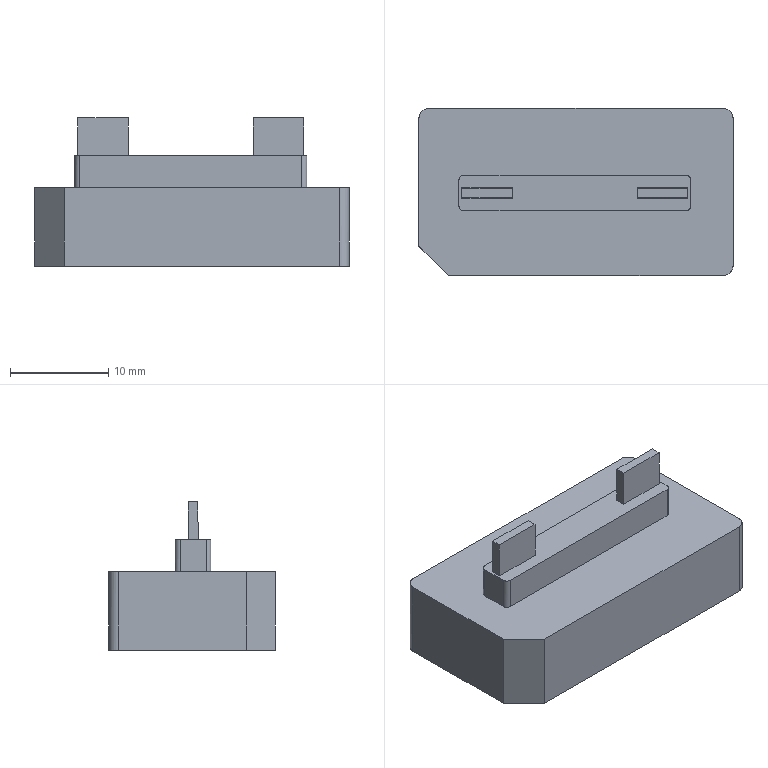NC program | PowerMill | posted by the shop | part box 32 x 17 x 15.109 mm
Lines 3804 to 5363 of 35413:
( TOOL ID   D3_2_1 )
( TOOL DIA. 3. TIP RAD 0 LENGTH 62.2 )
( Z = -7.279 )
T10 M6
T13
G91 G28 Z0
G0 G90 G54
M08
S18000 M3
X0 Y0 M8
G43 Z10.799 H10
X12.217 Y-2.308
Z.814
G1 Z-.386 F1200
X12.204 Y-2.248 F2000
X12.183 Y-2.19
X12.155 Y-2.136
X12.12 Y-2.086
X12.079 Y-2.04
X12.032 Y-1.999
X11.981 Y-1.965
X11.925 Y-1.938
X11.867 Y-1.919
X11.807 Y-1.907
X11.746 Y-1.902
X11.685 Y-1.906
X11.668 Y-1.908
X11.564 Y-1.924
X11.45 Y-1.935
X11.322 Y-1.939
X11.173
X6.36
X6.222 Y-1.936
X6.111 Y-1.929
X6.013 Y-1.916
X5.92 Y-1.896
X5.827 Y-1.869
X5.734 Y-1.833
X5.639 Y-1.788
X5.549 Y-1.737
X5.463 Y-1.68
X5.383 Y-1.617
X5.307 Y-1.547
X5.238 Y-1.472
X5.173 Y-1.392
X5.115 Y-1.306
X5.064 Y-1.216
X5.019 Y-1.121
X4.982 Y-1.024
X4.953 Y-.928
X4.932 Y-.831
X4.919 Y-.734
X4.914 Y-.639
X4.913 Y-.543
X4.911 Y.197
Y.353
X4.915 Y.461
X4.926 Y.565
X4.944 Y.666
X4.97 Y.764
X5.004 Y.86
X5.045 Y.954
X5.093 Y1.043
X5.147 Y1.13
X5.208 Y1.212
X5.276 Y1.29
X5.349 Y1.363
X5.429 Y1.43
X5.503 Y1.484
X5.576 Y1.529
X5.654 Y1.572
X5.727 Y1.607
X5.795 Y1.633
X5.896 Y1.666
X5.979 Y1.688
X6.053 Y1.7
X6.124 Y1.707
X6.194 Y1.713
X6.254 Y1.714
X7.073
X8.895 Y1.715
X10.37 Y1.714
X11.307 Y1.717
X11.419 Y1.715
X11.528 Y1.706
X11.633 Y1.69
X11.733 Y1.668
X11.829 Y1.638
X11.922 Y1.602
X12.015 Y1.557
X12.104 Y1.505
X12.189 Y1.446
X12.27 Y1.38
X12.345 Y1.309
X12.414 Y1.233
X12.477 Y1.151
X12.534 Y1.066
X12.583 Y.976
X12.625 Y.883
X12.66 Y.787
X12.689 Y.689
X12.709 Y.606
X12.719 Y.534
X12.722 Y.466
X12.728 Y.142
X12.729 Y-.253
X12.725 Y-.636
X12.721 Y-.731
X12.708 Y-.828
X12.687 Y-.924
X12.658 Y-1.021
X12.621 Y-1.117
X12.577 Y-1.212
X12.524 Y-1.304
X12.468 Y-1.388
X12.405 Y-1.467
X12.336 Y-1.543
X12.26 Y-1.613
X12.178 Y-1.678
X12.093 Y-1.736
X12.014 Y-1.781
X11.919 Y-1.828
X11.827 Y-1.864
X11.738 Y-1.892
X11.668 Y-1.908
X11.539 Y-1.926
X11.408 Y-1.936
X11.277 Y-1.939 Z-.387
X7.936 Z-.392
X6.283 Y-1.94 Z-.395
X6.175 Y-1.936
X6.068 Y-1.925 Z-.396
X5.964 Y-1.906
X5.862 Y-1.879
X5.764 Y-1.845
X5.669 Y-1.804
X5.578 Y-1.756 Z-.397
X5.492 Y-1.701
X5.41 Y-1.64
X5.333 Y-1.572
X5.26 Y-1.498
X5.193 Y-1.417
X5.131 Y-1.331 Z-.398
X5.087 Y-1.261
X5.049 Y-1.189
X5.015 Y-1.113
X4.982 Y-1.023
X4.952 Y-.92
X4.93 Y-.822 Z-.399
X4.917 Y-.732
X4.912 Y-.652
Y-.571
X4.911 Y.356 Z-.401
X4.915 Y.463
X4.926 Y.568
X4.945 Y.669
X4.971 Y.767
X5.005 Y.862 Z-.402
X5.046 Y.957
X5.095 Y1.049
X5.151 Y1.136
X5.213 Y1.219
X5.282 Y1.297
X5.356 Y1.369 Z-.403
X5.436 Y1.435
X5.52 Y1.496
X5.609 Y1.55
X5.698 Y1.596
X5.787 Y1.633 Z-.404
X5.876 Y1.661
X5.936 Y1.676
X5.989 Y1.688
X6.042 Y1.699
X6.095 Y1.709
X6.149 Y1.713
X6.202 Y1.714
X6.256
X6.879 Y1.715 Z-.405
X8.938 Z-.409
X10.77 Y1.716 Z-.412
X11.307 Y1.717 Z-.413
X11.417 Y1.715
X11.525 Y1.707 Z-.414
X11.629 Y1.691
X11.727 Y1.67
X11.821 Y1.641
X11.912 Y1.606
X12.004 Y1.563
X12.093 Y1.512 Z-.415
X12.179 Y1.454
X12.261 Y1.389
X12.334 Y1.321
X12.403 Y1.246
X12.467 Y1.164
X12.528 Y1.076 Z-.416
X12.563 Y1.016
X12.594 Y.954
X12.626 Y.88
X12.661 Y.788
X12.689 Y.692
X12.708 Y.609 Z-.417
X12.718 Y.538
X12.722 Y.469
X12.728 Y.169
X12.729 Y-.195 Z-.418
X12.726 Y-.636 Z-.419
X12.721 Y-.73
X12.708 Y-.826
X12.688 Y-.923
X12.659 Y-1.021
X12.622 Y-1.117 Z-.42
X12.577 Y-1.212
X12.525 Y-1.303
X12.467 Y-1.39
X12.403 Y-1.47
X12.335 Y-1.544
X12.259 Y-1.614 Z-.421
X12.178 Y-1.679
X12.092 Y-1.737
X12.002 Y-1.788
X11.908 Y-1.832
X11.812 Y-1.869 Z-.422
X11.713 Y-1.898
X11.668 Y-1.908
X11.539 Y-1.926
X11.409 Y-1.937
X11.278 Y-1.939 Z-.423
X8.198 Z-.428
X6.283 Y-1.941 Z-.431
X6.175 Y-1.937
X6.069 Y-1.925 Z-.432
X5.964 Y-1.906
X5.862 Y-1.879
X5.763 Y-1.845
X5.668 Y-1.803
X5.577 Y-1.755
X5.491 Y-1.701 Z-.433
X5.41 Y-1.64
X5.334 Y-1.574
X5.26 Y-1.498
X5.192 Y-1.417
X5.131 Y-1.332 Z-.434
X5.087 Y-1.262
X5.049 Y-1.189
X5.015 Y-1.112
X4.981 Y-1.021
X4.951 Y-.918
X4.929 Y-.819 Z-.435
X4.917 Y-.73
X4.912 Y-.648
X4.911 Y-.566
Y.079 Z-.436
X4.91 Y.214
X4.911 Y.365 Z-.437
X4.917 Y.481
X4.928 Y.585
X4.936 Y.637
X4.947 Y.681
X4.959 Y.725
X4.976 Y.779
X5.003 Y.853
X5.033 Y.929 Z-.438
X5.057 Y.983
X5.078 Y1.023
X5.102 Y1.062
X5.167 Y1.157
X5.233 Y1.242
X5.3 Y1.317
X5.372 Y1.384 Z-.439
X5.449 Y1.447
X5.532 Y1.503
X5.622 Y1.555
X5.72 Y1.603
X5.8 Y1.636
X5.881 Y1.663 Z-.44
X5.97 Y1.685
X6.067 Y1.701
X6.177 Y1.711
X6.308 Y1.716
X6.483 Z-.441
X6.697 Y1.715
X8.938 Z-.445
X10.76 Y1.716 Z-.448
X11.307 Y1.717 Z-.449
X11.417 Y1.715
X11.526 Y1.707
X11.63 Y1.692 Z-.45
X11.728 Y1.67
X11.822 Y1.641
X11.913 Y1.606
X12.005 Y1.563
X12.094 Y1.511 Z-.451
X12.18 Y1.453
X12.261 Y1.388
X12.335 Y1.32
X12.404 Y1.245
X12.469 Y1.163
X12.529 Y1.075 Z-.452
X12.563 Y1.015
X12.594 Y.953
X12.627 Y.879
X12.661 Y.787
X12.69 Y.691
X12.708 Y.608
X12.718 Y.537 Z-.453
X12.722 Y.468
X12.728 Y.168
X12.729 Y-.198 Z-.454
X12.726 Y-.636 Z-.455
X12.721 Y-.73
X12.708 Y-.826
X12.688 Y-.923
X12.659 Y-1.021
X12.622 Y-1.117
X12.577 Y-1.212 Z-.456
X12.525 Y-1.304
X12.467 Y-1.39
X12.404 Y-1.47
X12.335 Y-1.545
X12.259 Y-1.615 Z-.457
X12.178 Y-1.679
X12.092 Y-1.737
X12.002 Y-1.788
X11.908 Y-1.833
X11.812 Y-1.869
X11.713 Y-1.898 Z-.458
X11.668 Y-1.909
X11.539 Y-1.927
X11.409 Y-1.937
X11.278 Y-1.939
X8.194 Y-1.94 Z-.464
X6.283 Y-1.941 Z-.467
X6.175 Y-1.937
X6.068 Y-1.925
X5.964 Y-1.906 Z-.468
X5.862 Y-1.879
X5.763 Y-1.845
X5.668 Y-1.804
X5.577 Y-1.756
X5.491 Y-1.701 Z-.469
X5.41 Y-1.641
X5.335 Y-1.574
X5.261 Y-1.5
X5.195 Y-1.422
X5.138 Y-1.343
X5.089 Y-1.262 Z-.47
X5.038 Y-1.162
X4.996 Y-1.063
X4.962 Y-.966
X4.938 Y-.87
X4.921 Y-.776 Z-.471
X4.913 Y-.684
X4.912 Y-.593
X4.911 Y.079 Z-.472
X4.91 Y.216
X4.911 Y.367 Z-.473
X4.916 Y.484
X4.928 Y.589
X4.936 Y.637
X4.946 Y.68
X4.958 Y.723
X4.975 Y.777
X5.001 Y.85
X5.032 Y.927 Z-.474
X5.056 Y.981
X5.076 Y1.021
X5.099 Y1.059
X5.165 Y1.155
X5.231 Y1.24
X5.298 Y1.315
X5.369 Y1.383 Z-.475
X5.445 Y1.444
X5.528 Y1.501
X5.617 Y1.554
X5.715 Y1.601
X5.795 Y1.635
X5.876 Y1.662 Z-.476
X5.964 Y1.684
X6.061 Y1.7
X6.171 Y1.711
X6.3 Y1.716
X6.471 Z-.477
X6.568
X8.939 Y1.715 Z-.481
X10.779 Y1.717 Z-.484
X11.309 Y1.718 Z-.485
X11.42 Y1.715
X11.529 Y1.707
X11.633 Y1.691 Z-.486
X11.731 Y1.669
X11.825 Y1.641
X11.916 Y1.605
X12.008 Y1.561
X12.097 Y1.51
X12.183 Y1.452 Z-.487
X12.264 Y1.386
X12.338 Y1.318
X12.406 Y1.243
X12.471 Y1.16
X12.531 Y1.072 Z-.488
X12.565 Y1.012
X12.596 Y.95
X12.629 Y.875
X12.663 Y.782
X12.691 Y.686
X12.709 Y.604
X12.719 Y.534 Z-.489
X12.722 Y.465
X12.728 Y.163
X12.729 Y-.205 Z-.49
X12.726 Y-.636 Z-.491
X12.721 Y-.73
X12.708 Y-.826
X12.688 Y-.923
X12.659 Y-1.021
X12.622 Y-1.118
X12.577 Y-1.212 Z-.492
X12.525 Y-1.304
X12.467 Y-1.39
X12.404 Y-1.47
X12.335 Y-1.545
X12.259 Y-1.615
X12.178 Y-1.679 Z-.493
X12.092 Y-1.737
X12.002 Y-1.789
X11.908 Y-1.833
X11.812 Y-1.869
X11.714 Y-1.898 Z-.494
X11.668 Y-1.909
X11.539 Y-1.927
X11.409 Y-1.937
X11.279 Y-1.94
X7.607 Z-.501
X6.283 Z-.503
X6.171 Y-1.937
X6.067 Y-1.926
X5.969 Y-1.909 Z-.504
X5.873 Y-1.885
X5.776 Y-1.851
X5.681 Y-1.811
X5.589 Y-1.763
X5.5 Y-1.708
X5.416 Y-1.646 Z-.505
X5.338 Y-1.579
X5.265 Y-1.506
X5.199 Y-1.428
X5.14 Y-1.346
X5.089 Y-1.263 Z-.506
X5.038 Y-1.165
X4.996 Y-1.067
X4.963 Y-.97
X4.938 Y-.874
X4.921 Y-.779
X4.913 Y-.687 Z-.507
X4.911 Y-.595
X4.91 Y-.076 Z-.508
Y-.04
Y-.001
Y.049
X4.909 Y.112
Y.195
X4.911 Y.318
X4.913 Y.413
X4.917 Y.484 Z-.509
X4.92 Y.539
X4.925 Y.583
X4.93 Y.618
X4.939 Y.654
X4.975 Y.779
X5.01 Y.877
X5.046 Y.961
X5.086 Y1.037 Z-.51
X5.132 Y1.11
X5.194 Y1.197
X5.26 Y1.275
X5.33 Y1.347
X5.393 Y1.403
X5.466 Y1.459 Z-.511
X5.512 Y1.492
X5.546 Y1.514
X5.581 Y1.534
X5.628 Y1.559
X5.7 Y1.596
X5.748 Y1.617
X5.785 Y1.632
X5.824 Y1.644
X5.926 Y1.675 Z-.512
X6.004 Y1.694
X6.071 Y1.703
X6.138 Y1.71
X6.204 Y1.715
X6.264
X6.992 Y1.716 Z-.513
X8.876 Z-.517
X10.402 Y1.715 Z-.519
X11.307 Y1.718 Z-.521
X11.416 Y1.716
X11.524 Y1.708
X11.628 Y1.693
X11.727 Y1.671 Z-.522
X11.82 Y1.642
X11.912 Y1.607
X12.004 Y1.564
X12.094 Y1.513
X12.179 Y1.454 Z-.523
X12.261 Y1.389
X12.335 Y1.321
X12.404 Y1.246
X12.468 Y1.165
X12.528 Y1.076
X12.563 Y1.016 Z-.524
X12.594 Y.954
X12.626 Y.881
X12.661 Y.789
X12.69 Y.693
X12.708 Y.61
X12.718 Y.538
X12.722 Y.469 Z-.525
X12.728 Y.167
X12.729 Y-.201 Z-.526
X12.726 Y-.636
X12.721 Y-.73 Z-.527
X12.708 Y-.826
X12.688 Y-.924
X12.659 Y-1.021
X12.622 Y-1.118
X12.577 Y-1.213
X12.525 Y-1.304 Z-.528
X12.467 Y-1.39
X12.403 Y-1.471
X12.334 Y-1.546
X12.259 Y-1.616
X12.177 Y-1.68 Z-.529
X12.091 Y-1.738
X12.001 Y-1.789
X11.907 Y-1.833
X11.811 Y-1.87
X11.713 Y-1.899
X11.668 Y-1.909 Z-.53
X11.539 Y-1.927
X11.409 Y-1.938
X11.279 Y-1.94
X7.627 Z-.537
X6.283 Y-1.941 Z-.539
X6.171 Y-1.937
X6.067 Y-1.927
X5.969 Y-1.909
X5.873 Y-1.885 Z-.54
X5.775 Y-1.852
X5.68 Y-1.811
X5.588 Y-1.763
X5.5 Y-1.708
X5.416 Y-1.646 Z-.541
X5.338 Y-1.579
X5.265 Y-1.506
X5.199 Y-1.428
X5.14 Y-1.347
X5.089 Y-1.263
X5.038 Y-1.166 Z-.542
X4.996 Y-1.068
X4.963 Y-.971
X4.938 Y-.875
X4.921 Y-.78
X4.912 Y-.688
X4.911 Y-.596 Z-.543
X4.91 Y-.076 Z-.544
Y-.04
Y-.001
X4.909 Y.049
Y.112
Y.195
X4.911 Y.318
X4.913 Y.413
X4.916 Y.484 Z-.545
X4.92 Y.539
X4.924 Y.583
X4.93 Y.618
X4.938 Y.654
X4.975 Y.779
X5.009 Y.877
X5.045 Y.961
X5.086 Y1.037 Z-.546
X5.132 Y1.111
X5.194 Y1.197
X5.26 Y1.276
X5.33 Y1.348
X5.393 Y1.403
X5.466 Y1.459 Z-.547
X5.512 Y1.493
X5.546 Y1.514
X5.581 Y1.534
X5.628 Y1.56
X5.7 Y1.596
X5.748 Y1.617
X5.785 Y1.632
X5.823 Y1.644
X5.926 Y1.675
X6.004 Y1.694 Z-.548
X6.071 Y1.704
X6.138 Y1.71
X6.204 Y1.715
X6.264 Y1.716
X6.997 Z-.549
X8.876 Z-.553
X10.402 Z-.555
X11.307 Y1.718 Z-.557
X11.416 Y1.716
X11.524 Y1.708
X11.628 Y1.693
X11.727 Y1.671 Z-.558
X11.82 Y1.643
X11.912 Y1.607
X12.005 Y1.564
X12.094 Y1.513
X12.179 Y1.455
X12.261 Y1.39 Z-.559
X12.335 Y1.321
X12.404 Y1.247
X12.468 Y1.165
X12.528 Y1.077
X12.563 Y1.017
X12.594 Y.955 Z-.56
X12.627 Y.881
X12.661 Y.789
X12.69 Y.693
X12.708 Y.61
X12.718 Y.538
X12.722 Y.469
X12.728 Y.167 Z-.561
X12.729 Y-.202 Z-.562
X12.726 Y-.636
X12.721 Y-.73 Z-.563
X12.708 Y-.826
X12.688 Y-.924
X12.659 Y-1.021
X12.622 Y-1.118
X12.577 Y-1.213
X12.525 Y-1.304 Z-.564
X12.467 Y-1.391
X12.404 Y-1.471
X12.334 Y-1.546
X12.259 Y-1.616
X12.178 Y-1.68
X12.091 Y-1.738 Z-.565
X12.001 Y-1.79
X11.907 Y-1.834
X11.811 Y-1.87
X11.714 Y-1.899
X11.668 Y-1.909
X11.539 Y-1.928 Z-.566
X11.41 Y-1.938
X11.279 Y-1.94
X7.646 Z-.572
X6.283 Y-1.941 Z-.575
X6.171 Y-1.938
X6.067 Y-1.927
X5.969 Y-1.91
X5.873 Y-1.885 Z-.576
X5.775 Y-1.852
X5.68 Y-1.812
X5.588 Y-1.764
X5.5 Y-1.709
X5.416 Y-1.647
X5.337 Y-1.579 Z-.577
X5.265 Y-1.507
X5.199 Y-1.429
X5.139 Y-1.347
X5.089 Y-1.264
X5.038 Y-1.166 Z-.578
X4.996 Y-1.069
X4.963 Y-.971
X4.938 Y-.875
X4.921 Y-.781
X4.912 Y-.688
X4.911 Y-.596 Z-.579
X4.91 Y-.076
X4.909 Y-.04 Z-.58
Y-.001
Y.049
Y.112
Y.195
X4.91 Y.318
X4.913 Y.413
X4.916 Y.484
X4.92 Y.539 Z-.581
X4.924 Y.583
X4.929 Y.619
X4.938 Y.654
X4.974 Y.779
X5.009 Y.877
X5.045 Y.961
X5.086 Y1.038
X5.132 Y1.111 Z-.582
X5.194 Y1.198
X5.26 Y1.276
X5.33 Y1.348
X5.393 Y1.404
X5.466 Y1.46
X5.512 Y1.493 Z-.583
X5.546 Y1.515
X5.581 Y1.535
X5.628 Y1.56
X5.7 Y1.596
X5.748 Y1.618
X5.785 Y1.632
X5.823 Y1.644
X5.926 Y1.676
X6.004 Y1.694
X6.071 Y1.704 Z-.584
X6.138 Y1.711
X6.204 Y1.716
X6.264
X7.002 Z-.585
X8.876 Z-.588
X10.402 Z-.591
X11.307 Y1.719 Z-.593
X11.416 Y1.717
X11.524 Y1.708
X11.628 Y1.693
X11.727 Y1.671
X11.82 Y1.643 Z-.594
X11.912 Y1.608
X12.004 Y1.564
X12.094 Y1.513
X12.179 Y1.455
X12.261 Y1.39
X12.335 Y1.322 Z-.595
X12.404 Y1.247
X12.468 Y1.165
X12.528 Y1.077
X12.563 Y1.017
X12.594 Y.955
X12.627 Y.881 Z-.596
X12.661 Y.789
X12.69 Y.693
X12.708 Y.61
X12.718 Y.538
X12.722 Y.469
X12.728 Y.166 Z-.597
X12.729 Y-.203 Z-.598
X12.726 Y-.636
X12.721 Y-.73
X12.708 Y-.827 Z-.599
X12.688 Y-.924
X12.659 Y-1.022
X12.622 Y-1.118
X12.577 Y-1.213
X12.525 Y-1.304
X12.467 Y-1.391 Z-.6
X12.404 Y-1.471
X12.334 Y-1.546
X12.259 Y-1.616
X12.178 Y-1.681
X12.091 Y-1.739 Z-.601
X12.001 Y-1.79
X11.907 Y-1.834
X11.812 Y-1.871
X11.714 Y-1.899
X11.668 Y-1.91
X11.54 Y-1.928 Z-.602
X11.41 Y-1.938
X11.28 Y-1.941
X7.664 Z-.608
X6.283 Z-.611
X6.171 Y-1.938
X6.066 Y-1.927
X5.969 Y-1.91
X5.873 Y-1.886
X5.775 Y-1.853 Z-.612
X5.68 Y-1.812
X5.588 Y-1.764
X5.5 Y-1.709
X5.416 Y-1.647
X5.337 Y-1.58 Z-.613
X5.265 Y-1.507
X5.199 Y-1.429
X5.139 Y-1.348
X5.089 Y-1.265
X5.038 Y-1.167
X4.996 Y-1.07 Z-.614
X4.963 Y-.972
X4.937 Y-.876
X4.921 Y-.782
X4.912 Y-.689
X4.91 Y-.597
X4.909 Y-.076 Z-.615
Y-.04
Y-.001
Y.049 Z-.616
X4.908 Y.112
X4.909 Y.195
X4.91 Y.318
X4.912 Y.413
X4.916 Y.484
X4.919 Y.539
X4.924 Y.583 Z-.617
X4.929 Y.619
X4.938 Y.654
X4.974 Y.779
X5.008 Y.877
X5.045 Y.962
X5.085 Y1.038
X5.132 Y1.112 Z-.618
X5.194 Y1.198
X5.26 Y1.277
X5.33 Y1.349
X5.393 Y1.404
X5.465 Y1.46
X5.512 Y1.494
X5.546 Y1.515 Z-.619
X5.581 Y1.535
X5.628 Y1.561
X5.7 Y1.597
X5.748 Y1.618
X5.785 Y1.633
X5.823 Y1.645
X5.926 Y1.676
X6.004 Y1.695
X6.071 Y1.704
X6.138 Y1.711 Z-.62
X6.204 Y1.716
X6.264
X7.008 Y1.717 Z-.621
X8.876 Z-.624
X10.402 Y1.716 Z-.627
X11.307 Y1.719 Z-.629
X11.416 Y1.717
X11.524 Y1.709
X11.628 Y1.694
X11.727 Y1.672
X11.821 Y1.643 Z-.63
X11.912 Y1.608
X12.005 Y1.564
X12.094 Y1.513
X12.179 Y1.455
X12.261 Y1.39
X12.335 Y1.322 Z-.631
X12.404 Y1.247
X12.468 Y1.165
X12.528 Y1.077
X12.563 Y1.017
X12.594 Y.955
X12.627 Y.881 Z-.632
X12.661 Y.789
X12.69 Y.693
X12.708 Y.609
X12.719 Y.538
X12.722 Y.469
X12.728 Y.165 Z-.633
X12.729 Y-.205
X12.726 Y-.636 Z-.634
X12.721 Y-.73
X12.708 Y-.827
X12.688 Y-.924 Z-.635
X12.659 Y-1.022
X12.622 Y-1.119
X12.577 Y-1.213
X12.525 Y-1.305
X12.467 Y-1.391 Z-.636
X12.404 Y-1.472
X12.334 Y-1.547
X12.259 Y-1.617
X12.177 Y-1.681
X12.091 Y-1.739
X12.001 Y-1.79 Z-.637
X11.907 Y-1.834
X11.812 Y-1.871
X11.714 Y-1.899
X11.669 Y-1.91
X11.54 Y-1.928
X11.41 Y-1.938 Z-.638
X11.28 Y-1.941
X7.683 Z-.644
X6.283 Y-1.942 Z-.647
X6.171 Y-1.938
X6.066 Y-1.928
X5.968 Y-1.911
X5.873 Y-1.886
X5.775 Y-1.853 Z-.648
X5.68 Y-1.812
X5.588 Y-1.764
X5.5 Y-1.709
X5.416 Y-1.648
X5.337 Y-1.58
X5.265 Y-1.507 Z-.649
X5.198 Y-1.43
X5.139 Y-1.348
X5.089 Y-1.266
X5.038 Y-1.168
X4.996 Y-1.071 Z-.65
X4.962 Y-.973
X4.937 Y-.877
X4.92 Y-.783
X4.912 Y-.69
X4.91 Y-.598
X4.909 Y-.076 Z-.651
Y-.04
Y-.001
X4.908 Y.049
Y.112 Z-.652
Y.195
X4.91 Y.318
X4.912 Y.413
X4.915 Y.484
X4.919 Y.539
X4.923 Y.583
X4.929 Y.619
X4.937 Y.654 Z-.653
X4.973 Y.778
X5.008 Y.877
X5.044 Y.962
X5.085 Y1.038
X5.131 Y1.112
X5.194 Y1.198 Z-.654
X5.259 Y1.277
X5.33 Y1.349
X5.393 Y1.405
X5.465 Y1.46
X5.512 Y1.494
X5.546 Y1.516
X5.581 Y1.536
X5.628 Y1.561 Z-.655
X5.7 Y1.597
X5.747 Y1.619
X5.784 Y1.633
X5.823 Y1.645
X5.926 Y1.676
X6.004 Y1.695
X6.071 Y1.705
X6.137 Y1.711 Z-.656
X6.204 Y1.716
X6.264 Y1.717
X7.013 Z-.657
X8.876 Z-.66
X10.402 Z-.663
X11.307 Y1.719 Z-.665
X11.416 Y1.717
X11.524 Y1.709
X11.628 Y1.694
X11.727 Y1.672
X11.821 Y1.644
X11.912 Y1.608 Z-.666
X12.005 Y1.565
X12.094 Y1.514
X12.179 Y1.456
X12.261 Y1.391
X12.335 Y1.322
X12.404 Y1.247 Z-.667
X12.468 Y1.166
X12.528 Y1.077
X12.563 Y1.017
X12.594 Y.955
X12.627 Y.881
X12.661 Y.79 Z-.668
X12.69 Y.693
X12.708 Y.61
X12.719 Y.538
X12.722 Y.469
X12.728 Y.165 Z-.669
X12.729 Y-.206
X12.726 Y-.636 Z-.67
X12.721 Y-.731
X12.708 Y-.827
X12.688 Y-.924 Z-.671
X12.659 Y-1.022
X12.622 Y-1.119
X12.577 Y-1.213
X12.526 Y-1.305
X12.467 Y-1.391
X12.404 Y-1.472 Z-.672
X12.334 Y-1.547
X12.259 Y-1.617
X12.177 Y-1.681
X12.091 Y-1.739
X12.001 Y-1.791 Z-.673
X11.907 Y-1.835
X11.812 Y-1.871
X11.715 Y-1.9
X11.669 Y-1.91
X11.54 Y-1.928
X11.41 Y-1.939 Z-.674
X11.28 Y-1.941
X7.7 Z-.68
X6.283 Y-1.942 Z-.683
X6.171 Y-1.939
X6.066 Y-1.928
X5.968 Y-1.911
X5.873 Y-1.886
X5.775 Y-1.853
X5.68 Y-1.813 Z-.684
X5.588 Y-1.765
X5.499 Y-1.71
X5.415 Y-1.648
X5.337 Y-1.581
X5.264 Y-1.508 Z-.685
X5.198 Y-1.43
X5.139 Y-1.349
X5.089 Y-1.267
X5.038 Y-1.169
X4.996 Y-1.071
X4.962 Y-.974 Z-.686
X4.937 Y-.878
X4.92 Y-.783
X4.911 Y-.69
X4.91 Y-.598
X4.909 Y-.076 Z-.687
Y-.04
X4.908 Y-.001
Y.049
Y.112 Z-.688
Y.195
X4.909 Y.318
X4.912 Y.413
X4.915 Y.484
X4.919 Y.539
X4.923 Y.583
X4.928 Y.619
X4.937 Y.654
X4.973 Y.778 Z-.689
X5.007 Y.877
X5.044 Y.962
X5.085 Y1.039
X5.131 Y1.113
X5.193 Y1.198 Z-.69
X5.257 Y1.276
X5.325 Y1.346
X5.399 Y1.41
X5.485 Y1.475
X5.55 Y1.519
X5.618 Y1.558
X5.703 Y1.599 Z-.691
X5.776 Y1.63
X5.843 Y1.653
X5.935 Y1.681
X6.013 Y1.698
X6.078 Y1.706
X6.163 Y1.714
X6.224 Y1.717 Z-.692
X6.964 Z-.693
X8.877 Z-.696
X10.292 Z-.699
X11.25 Y1.72 Z-.7
X11.366 Z-.701
X11.479 Y1.714
X11.586 Y1.701
X11.689 Y1.681
X11.789 Y1.654
X11.884 Y1.62
X11.977 Y1.579 Z-.702
X12.066 Y1.531
X12.152 Y1.476
X12.234 Y1.414
X12.312 Y1.344
X12.385 Y1.27 Z-.703
X12.45 Y1.192
X12.508 Y1.11
X12.558 Y1.025
X12.602 Y.938
X12.644 Y.838
X12.677 Y.744 Z-.704
X12.7 Y.654
X12.715 Y.569
X12.721 Y.488
X12.728 Y.223
X12.73 Y-.096 Z-.705
X12.726 Y-.562 Z-.706
X12.725 Y-.656
X12.719 Y-.75
X12.705 Y-.847
X12.683 Y-.944 Z-.707
X12.652 Y-1.041
X12.614 Y-1.138
X12.568 Y-1.232
X12.515 Y-1.322
X12.455 Y-1.408
X12.392 Y-1.486 Z-.708
X12.321 Y-1.56
X12.245 Y-1.629
X12.163 Y-1.692
X12.076 Y-1.749
X11.985 Y-1.799
X11.891 Y-1.842 Z-.709
X11.795 Y-1.877
X11.698 Y-1.904
X11.669 Y-1.91
X11.54 Y-1.929
X11.41 Y-1.939 Z-.71
X11.28 Y-1.942
X7.718 Z-.716
X6.283 Z-.718
X6.171 Y-1.939 Z-.719
X6.066 Y-1.928
X5.968 Y-1.911
X5.873 Y-1.887
X5.775 Y-1.854
X5.68 Y-1.813 Z-.72
X5.588 Y-1.765
X5.499 Y-1.71
X5.415 Y-1.648
X5.337 Y-1.581
X5.264 Y-1.508
X5.198 Y-1.431 Z-.721
X5.139 Y-1.349
X5.089 Y-1.268
X5.038 Y-1.17
X4.996 Y-1.072
X4.962 Y-.975 Z-.722
X4.937 Y-.879
X4.92 Y-.784
X4.911 Y-.691
X4.909 Y-.599
X4.908 Y-.076 Z-.723
Y-.04
Y-.001
Y.048
X4.907 Y.111
X4.908 Y.194 Z-.724
X4.909 Y.316
X4.911 Y.412
X4.915 Y.483
X4.918 Y.538
X4.922 Y.582
X4.928 Y.618
X4.936 Y.653
X4.972 Y.777 Z-.725
X5.007 Y.877
X5.043 Y.962
X5.084 Y1.037
X5.129 Y1.11
X5.192 Y1.198
X5.256 Y1.276 Z-.726
X5.323 Y1.345
X5.394 Y1.407
X5.48 Y1.473
X5.567 Y1.529
X5.655 Y1.577
X5.743 Y1.618 Z-.727
X5.822 Y1.647
X5.902 Y1.671
X5.985 Y1.69
X6.074 Y1.705
X6.176 Y1.715
X6.296 Y1.719 Z-.728
X6.404
X6.509
X7.67 Y1.717 Z-.73
X9.612 Y1.718 Z-.733
X10.654 Z-.735
X11.307 Y1.72 Z-.736
X11.423 Y1.718 Z-.737
X11.533 Y1.708
X11.639 Y1.692
X11.74 Y1.668
X11.837 Y1.638
X11.931 Y1.6
X12.021 Y1.557 Z-.738
X12.108 Y1.505
X12.192 Y1.447
X12.272 Y1.381
X12.348 Y1.309
X12.417 Y1.233 Z-.739
X12.479 Y1.153
X12.533 Y1.069
X12.579 Y.985
X12.627 Y.882
X12.663 Y.786
X12.691 Y.694 Z-.74
X12.709 Y.607
X12.719 Y.524
X12.723 Y.442
X12.729 Y.17
Y-.164 Z-.741
X12.726 Y-.636 Z-.742
X12.721 Y-.73
X12.709 Y-.826
X12.688 Y-.923
X12.66 Y-1.021 Z-.743
X12.623 Y-1.117
X12.578 Y-1.212
X12.527 Y-1.304
X12.468 Y-1.39
X12.405 Y-1.471
X12.336 Y-1.546 Z-.744
X12.261 Y-1.615
X12.18 Y-1.68
X12.093 Y-1.739
X12.003 Y-1.79
X11.91 Y-1.834 Z-.745
X11.815 Y-1.871
X11.719 Y-1.899
X11.669 Y-1.911
X11.54 Y-1.929
X11.411 Y-1.939
X11.281 Y-1.942 Z-.746
X8.41 Z-.751
X6.283 Y-1.943 Z-.754
X6.175 Y-1.94 Z-.755
X6.068 Y-1.928
X5.964 Y-1.909
X5.862 Y-1.882
X5.764 Y-1.848
X5.668 Y-1.807
X5.577 Y-1.759 Z-.756
X5.489 Y-1.704
X5.407 Y-1.642
X5.329 Y-1.574
X5.257 Y-1.501
X5.191 Y-1.423 Z-.757
X5.133 Y-1.341
X5.081 Y-1.255
X5.032 Y-1.157
X4.991 Y-1.06
X4.958 Y-.963
X4.934 Y-.867 Z-.758
X4.918 Y-.772
X4.91 Y-.679
X4.909 Y-.587
X4.908 Y-.076 Z-.759
Y-.04
Y-.001
X4.907 Y.048
Y.112
Y.194
X4.909 Y.316 Z-.76
X4.911 Y.412
X4.914 Y.483
X4.918 Y.538
X4.922 Y.582
X4.927 Y.618
X4.936 Y.653
X4.972 Y.777
X5.006 Y.877 Z-.761
X5.043 Y.962
X5.083 Y1.038
X5.129 Y1.111
X5.191 Y1.198
X5.256 Y1.276
X5.323 Y1.345 Z-.762
X5.394 Y1.408
X5.48 Y1.473
X5.567 Y1.53
X5.655 Y1.578
X5.743 Y1.618 Z-.763
X5.822 Y1.647
X5.902 Y1.671
X5.985 Y1.691
X6.074 Y1.705
X6.176 Y1.715
X6.296 Y1.719 Z-.764
X6.404 Y1.72
X6.51 Y1.719
X7.671 Y1.717 Z-.766
X9.614 Y1.718 Z-.769
X10.656 Z-.771
X11.307 Y1.721 Z-.772
X11.423 Y1.718
X11.533 Y1.709 Z-.773
X11.639 Y1.692
X11.74 Y1.669
X11.837 Y1.638
X11.931 Y1.601
X12.021 Y1.557 Z-.774
X12.108 Y1.506
X12.192 Y1.447
X12.272 Y1.382
X12.348 Y1.31
X12.417 Y1.233
X12.479 Y1.153 Z-.775
X12.533 Y1.07
X12.579 Y.986
X12.627 Y.883
X12.663 Y.786
X12.691 Y.695
X12.709 Y.608 Z-.776
X12.719 Y.524
X12.723 Y.442
X12.729 Y.17
Y-.164 Z-.777
X12.726 Y-.636 Z-.778
X12.721 Y-.73
X12.709 Y-.826
X12.688 Y-.923
X12.66 Y-1.021
X12.623 Y-1.117 Z-.779
X12.578 Y-1.212
X12.527 Y-1.304
X12.468 Y-1.391
X12.405 Y-1.472
X12.336 Y-1.546 Z-.78
X12.261 Y-1.616
X12.18 Y-1.68
X12.093 Y-1.739
X12.003 Y-1.791
X11.91 Y-1.835
X11.815 Y-1.871 Z-.781
X11.719 Y-1.899
X11.669 Y-1.911
X11.54 Y-1.929
X11.411 Y-1.94
X11.281 Y-1.942 Z-.782
X8.42 Y-1.943 Z-.787
X6.283 Y-1.944 Z-.79
X6.175 Y-1.94
X6.068 Y-1.929 Z-.791
X5.964 Y-1.909
X5.862 Y-1.883
X5.763 Y-1.849
X5.668 Y-1.807
X5.576 Y-1.759 Z-.792
X5.489 Y-1.704
X5.407 Y-1.643
X5.329 Y-1.575
X5.257 Y-1.502
X5.191 Y-1.424
X5.133 Y-1.342 Z-.793
X5.082 Y-1.257
X5.032 Y-1.158
X4.99 Y-1.06
X4.958 Y-.963
X4.933 Y-.868 Z-.794
X4.917 Y-.774
X4.909 Y-.682
X4.908 Y-.59
Y-.076 Z-.795
Y-.04
X4.907 Y-.001
Y.048
Y.112
Y.194
X4.909 Y.317 Z-.796
X4.911 Y.412
X4.914 Y.483
X4.918 Y.539
X4.922 Y.582
X4.927 Y.618
X4.936 Y.654
X4.971 Y.777
X5.006 Y.877 Z-.797
X5.044 Y.965
X5.085 Y1.042
X5.131 Y1.116
X5.194 Y1.203
X5.26 Y1.281
X5.329 Y1.351 Z-.798
X5.403 Y1.415
X5.487 Y1.479
X5.574 Y1.535
X5.663 Y1.582
X5.754 Y1.622
X5.833 Y1.651 Z-.799
X5.913 Y1.674
X5.996 Y1.693
X6.086 Y1.707
X6.19 Y1.716
X6.309 Y1.72
X6.416 Z-.8
X6.523 Y1.719
X7.689 Y1.718 Z-.802
X9.633 Z-.805
X10.675 Y1.719 Z-.807
X11.307 Y1.721 Z-.808
X11.423 Y1.718
X11.533 Y1.709 Z-.809
X11.639 Y1.692
X11.74 Y1.669
X11.837 Y1.639
X11.931 Y1.601
X12.021 Y1.557
X12.108 Y1.506 Z-.81
X12.192 Y1.448
X12.272 Y1.382
X12.348 Y1.31
X12.417 Y1.234
X12.479 Y1.153
X12.533 Y1.07 Z-.811
X12.579 Y.986
X12.627 Y.883
X12.663 Y.786
X12.691 Y.695
X12.709 Y.608 Z-.812
X12.719 Y.525
X12.723 Y.442
X12.729 Y.17
Y-.165 Z-.813
X12.726 Y-.636 Z-.814
X12.721 Y-.73
X12.709 Y-.826
X12.688 Y-.923
X12.66 Y-1.021
X12.623 Y-1.118 Z-.815
X12.579 Y-1.212
X12.527 Y-1.304
X12.469 Y-1.391
X12.405 Y-1.472
X12.336 Y-1.546
X12.261 Y-1.616 Z-.816
X12.18 Y-1.681
X12.094 Y-1.739
X12.003 Y-1.791
X11.91 Y-1.835
X11.815 Y-1.871 Z-.817
X11.719 Y-1.9
X11.669 Y-1.911
X11.54 Y-1.93
X11.411 Y-1.94
X11.281 Y-1.943
X8.429 Z-.822
X6.283 Y-1.944 Z-.826
X6.175 Y-1.94
X6.068 Y-1.929 Z-.827
X5.964 Y-1.91
X5.862 Y-1.883
X5.763 Y-1.849
X5.668 Y-1.808
X5.576 Y-1.76
X5.489 Y-1.705 Z-.828
X5.406 Y-1.643
X5.329 Y-1.575
X5.257 Y-1.502
X5.191 Y-1.424
X5.133 Y-1.342 Z-.829
X5.081 Y-1.257
X5.031 Y-1.159
X4.99 Y-1.061
X4.957 Y-.964
X4.933 Y-.868
X4.917 Y-.774 Z-.83
X4.909 Y-.682
X4.908 Y-.59
Y-.076 Z-.831
X4.907 Y-.04
Y-.001
Y.048
Y.112
Y.195
X4.908 Y.317
X4.911 Y.412 Z-.832
X4.914 Y.483
X4.917 Y.539
X4.922 Y.582
X4.927 Y.618
X4.935 Y.654
X4.971 Y.777
X5.006 Y.877
X5.043 Y.965 Z-.833
X5.084 Y1.042
X5.131 Y1.116
X5.194 Y1.203
X5.26 Y1.281
X5.329 Y1.352
X5.402 Y1.415 Z-.834
X5.487 Y1.479
X5.574 Y1.535
X5.663 Y1.583
X5.753 Y1.623
X5.832 Y1.651 Z-.835
X5.912 Y1.675
X5.995 Y1.694
X6.086 Y1.708
X6.19 Y1.717
X6.309 Y1.72
X6.416 Z-.836
X6.523
X7.691 Y1.718 Z-.838
X9.637 Y1.719 Z-.841
X10.689 Z-.843
X11.309 Y1.721 Z-.844
X11.425 Y1.718
X11.535 Y1.709
X11.641 Y1.692 Z-.845
X11.742 Y1.669
X11.839 Y1.638
X11.933 Y1.601
X12.023 Y1.556
X12.11 Y1.505 Z-.846
X12.194 Y1.446
X12.274 Y1.381
X12.35 Y1.309
X12.419 Y1.232
X12.48 Y1.152
X12.535 Y1.068 Z-.847
X12.579 Y.986
X12.627 Y.883
X12.663 Y.787
X12.691 Y.695
X12.709 Y.608
X12.719 Y.525 Z-.848
X12.723 Y.443
X12.729 Y.17
Y-.166 Z-.849
X12.726 Y-.636 Z-.85
X12.721 Y-.73
X12.709 Y-.826
X12.688 Y-.924
X12.66 Y-1.021
X12.623 Y-1.118
X12.579 Y-1.213 Z-.851
X12.527 Y-1.304
X12.469 Y-1.391
X12.405 Y-1.472
X12.336 Y-1.546
X12.261 Y-1.616 Z-.852
X12.18 Y-1.681
X12.094 Y-1.739
X12.003 Y-1.791
X11.91 Y-1.835
X11.815 Y-1.871
X11.72 Y-1.9 Z-.853
X11.669 Y-1.911
X11.541 Y-1.93
X11.411 Y-1.94
X11.282 Y-1.943
X8.439 Z-.858
X6.283 Y-1.944 Z-.862
X6.174 Y-1.941
X6.068 Y-1.929
X5.964 Y-1.91 Z-.863
X5.862 Y-1.884
X5.763 Y-1.849
X5.668 Y-1.808
X5.576 Y-1.76
X5.489 Y-1.705 Z-.864
X5.406 Y-1.643
X5.328 Y-1.576
X5.256 Y-1.502
X5.191 Y-1.425
X5.132 Y-1.343
X5.081 Y-1.257 Z-.865
X5.031 Y-1.159
X4.99 Y-1.061
X4.957 Y-.964
X4.933 Y-.869
X4.917 Y-.774
X4.909 Y-.682 Z-.866
X4.908 Y-.59
X4.907 Y-.076 Z-.867
Y-.04
Y-.001
Y.048
X4.906 Y.112
X4.907 Y.195
X4.908 Y.317
X4.91 Y.413 Z-.868
X4.913 Y.483
X4.917 Y.539
X4.921 Y.582
X4.926 Y.618
X4.935 Y.654
X4.97 Y.776
X5.005 Y.877
X5.043 Y.964 Z-.869
X5.084 Y1.042
X5.13 Y1.116
X5.193 Y1.202
X5.258 Y1.281
X5.327 Y1.351
X5.4 Y1.414 Z-.87
X5.485 Y1.478
X5.572 Y1.534
X5.66 Y1.582